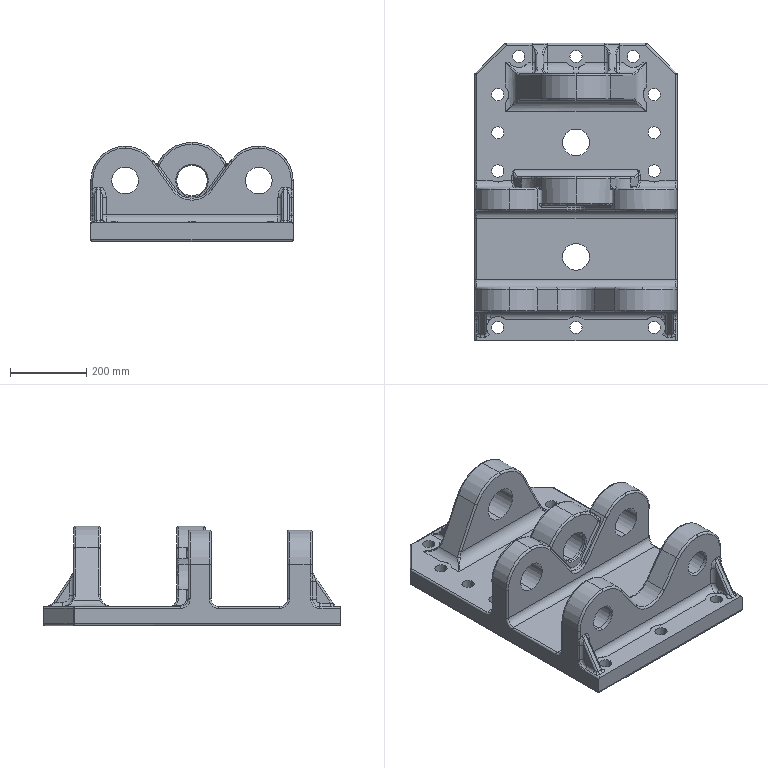Part | SolidWorks | features Fillet 26, ICE 14, Chamfer 4, MirrorPattern 3, 3DProfileFeature 2, HoleWzd 2, LPattern 2, Extrusion 1 | 1 solid | 408 faces | box 530 x 780 x 260 mm | volume 33233633 mm3 | cylinder 197 | cone 58 | torus 49 | spline 47 | plane 45 | sphere 12 | commonest cylinder face diameters 10 x69 32 x24 10.2 x20 20 x20 58 x12 60 x10